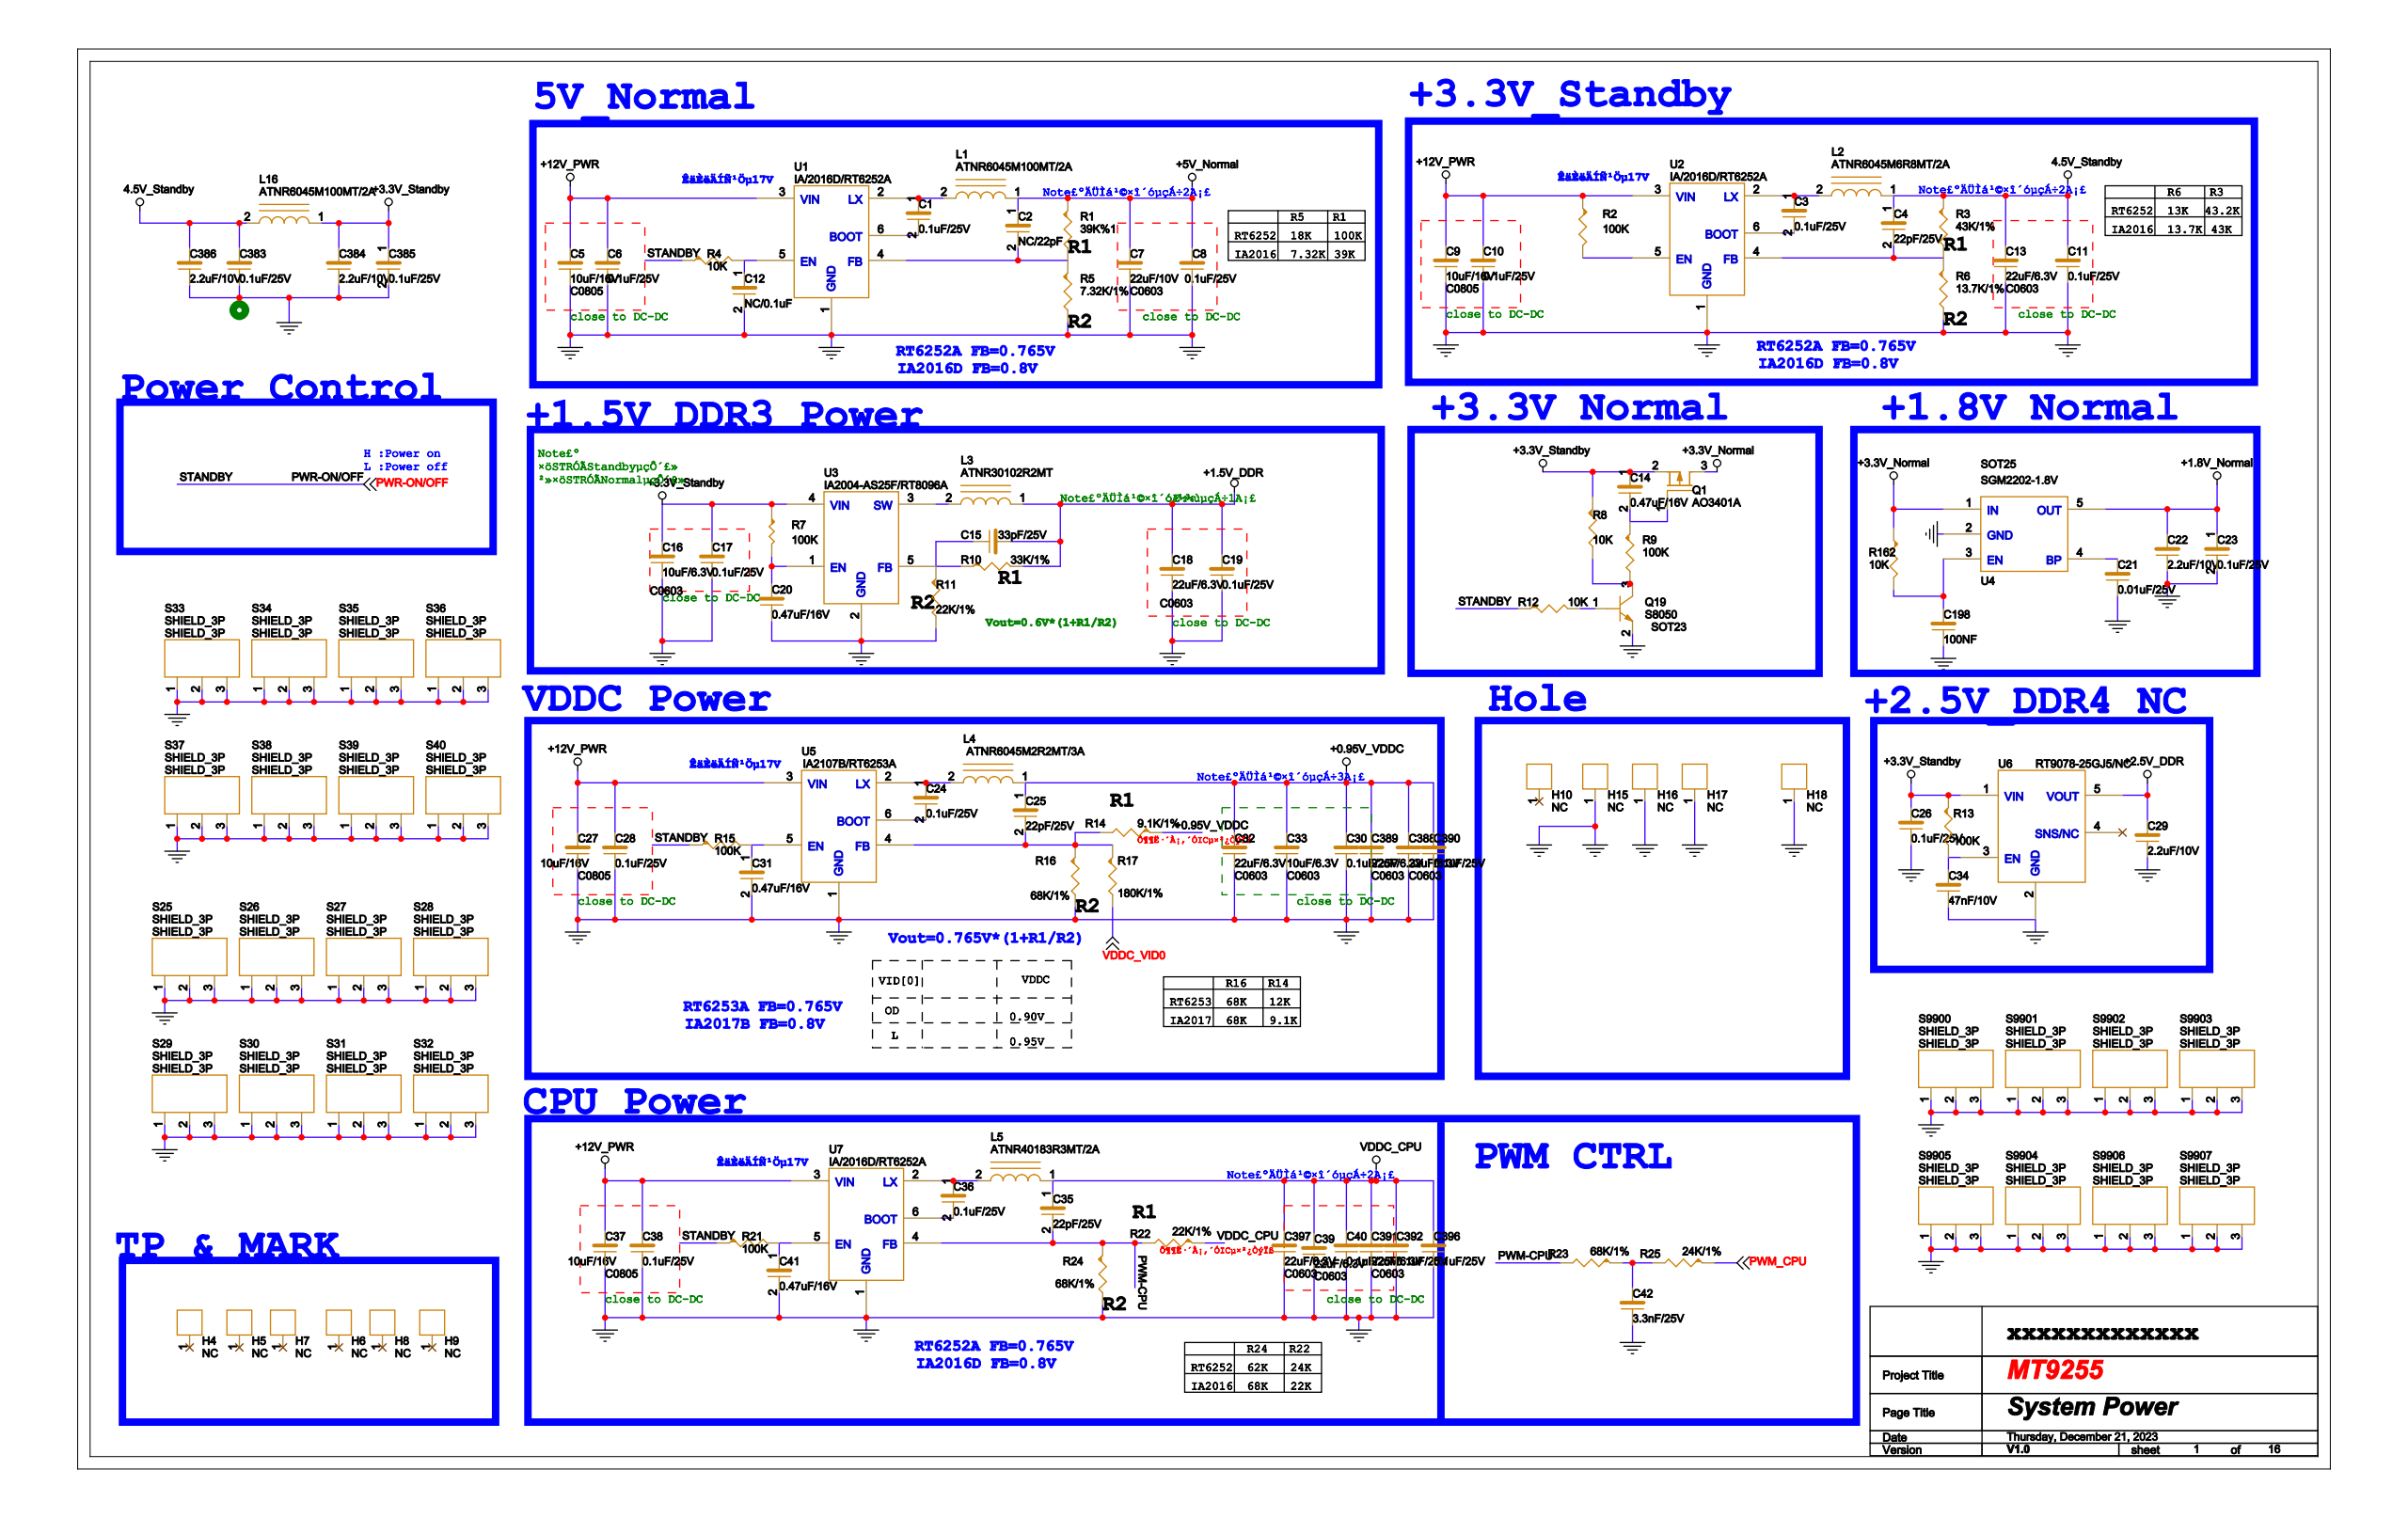Circuit board | Cadence Allegro | 1223 parts | 777 nets | one sheet of the schematic
Parts on this sheet (reference | value | footprint):
C2 | NC/22pF | C0402
C4 | 22pF/25V | C0402
C5 | 10uF/16V | C0805
C6 | 0.1uF/25V | C0402
C7 | 22uF/10V | C0603
C9 | 10uF/16V | C0805
C10 | 0.1uF/25V | C0402
C12 | NC/0.1uF | C0402
C15 | 33pF/25V | C0402
C17 | 0.1uF/25V | C0402
C18 | 22uF/6.3V | C0603
C19 | 0.1uF/25V | C0402
C20 | 0.47uF/16V | C0402
C21 | 0.01uF/25V | C0402
C25 | 22pF/25V | C0402
C26 | 0.1uF/25V | C0402
C27 | 10uF/16V | C0805
C28 | 0.1uF/25V | C0402
C29 | 2.2uF/10V | C0402
C30 | 0.1uF/25V | C0402
C31 | 0.47uF/16V | C0402
C32 | 22uF/6.3V | C0603
C33 | 10uF/6.3V | C0603
C34 | 47nF/10V | C0402
C35 | 22pF/25V | C0402
C36 | 0.1uF/25V | C0402
C37 | 10uF/16V | C0805
C38 | 0.1uF/25V | C0402
C39 | 22uF/6.3V | C0603
C40 | 0.1uF/25V | C0402
C41 | 0.47uF/16V | C0402
C42 | 3.3nF/25V | C0402
C198 | 100NF | C0402
C383 | 0.1uF/25V | C0402
C384 | 2.2uF/10V | C0402
C385 | 0.1uF/25V | C0402
C386 | 2.2uF/10V | C0402
C388 | 22uF/6.3V | C0603
C389 | 22uF/6.3V | C0603
C390 | 0.1uF/25V | C0402
C391 | 22uF/6.3V | C0603
C392 | 0.1uF/25V | C0402
C396 | 0.1uF/25V | C0402
C397 | 22uF/6.3V | C0603
H15 | NC | HOLE_D1D8MM
H16 | NC | HOLE_D1D8MM
H17 | NC | HOLE_D1D8MM
H18 | NC | HOLE_D1D8MM
L1 | ATNR6045M100MT/2A | MWSA0402S
L2 | ATNR6045M6R8MT/2A | MWSA0402S
L3 | ATNR30102R2MT | SMD03X03
L4 | ATNR6045M2R2MT/3A | MWSA0402S
L5 | ATNR40183R3MT/2A | MWSA0402S
L16 | ATNR6045M100MT/2A | MWSA0402S
Q1 | AO3401A | SOT23-100
Q19 | S8050 | SOT23
R3 | 43K/1% | R0402
R4 | 10K | R0402
R6 | 13.7K/1% | R0402
R7 | 100K | R0402
R10 | 33K/1% | R0402
R11 | 22K/1% | R0402
R12 | 10K | R0402
R14 | 9.1K/1% | R0402
R15 | 100K | R0402
R16 | 68K/1% | R0402
R17 | 180K/1% | R0402
R21 | 100K | R0402
R22 | 22K/1% | R0402
R23 | 68K/1% | R0402
R24 | 68K/1% | R0402
R25 | 24K/1% | R0402
R162 | 10K | R0402
S25 | SHIELD_3P | SHIELD_3P
S26 | SHIELD_3P | SHIELD_3P
S27 | SHIELD_3P | SHIELD_3P
S28 | SHIELD_3P | SHIELD_3P
S29 | SHIELD_3P | SHIELD_3P
S30 | SHIELD_3P | SHIELD_3P
S31 | SHIELD_3P | SHIELD_3P
S32 | SHIELD_3P | SHIELD_3P
S33 | SHIELD_3P | SHIELD_3P
S34 | SHIELD_3P | SHIELD_3P
S35 | SHIELD_3P | SHIELD_3P
S36 | SHIELD_3P | SHIELD_3P
S37 | SHIELD_3P | SHIELD_3P
S38 | SHIELD_3P | SHIELD_3P
S39 | SHIELD_3P | SHIELD_3P
S40 | SHIELD_3P | SHIELD_3P
S9900 | SHIELD_3P | SHIELD_3P
S9901 | SHIELD_3P | SHIELD_3P
S9902 | SHIELD_3P | SHIELD_3P
S9903 | SHIELD_3P | SHIELD_3P
S9904 | SHIELD_3P | SHIELD_3P
S9905 | SHIELD_3P | SHIELD_3P
S9906 | SHIELD_3P | SHIELD_3P
S9907 | SHIELD_3P | SHIELD_3P
U1 | IA/2016D/RT6252A | SOT-23-6
U2 | IA/2016D/RT6252A | SOT-23-6
U3 | IA2004-AS25F/RT8096A | SOT25
U4 | SGM2202-1.8V | SOT25
U5 | IA2107B/RT6253A | SOT-23-6
U6 | RT9078-25GJ5/NC | SOT25
U7 | IA/2016D/RT6252A | SOT-23-6
Nets of these parts (net: part-pin ...):
GND: C5-2 C6-2 C7-2 C9-2 C10-2 C12-2 C17-2 C18-2 C19-2 C20-2 C21-2 C26-2 C27-2 C28-2 C29-2 C30-2 C31-2 C32-2 C33-2 C34-2 C37-2 C38-2 C39-2 C40-2 C41-2 C42-2 C198-2 C383-2 C384-2 C385-2 C386-2 C388-2 C389-2 C390-2 C391-2 C392-2 C396-2 C397-2 H15-1 H16-1 H17-1 H18-1 Q19-2 R6-2 R11-2 R16-2 R24-2 S25-1 S25-2 S25-3 S26-1 S26-2 S26-3 S27-1 S27-2 S27-3 S28-1 S28-2 S28-3 S29-1 S29-2 S29-3 S30-1 S30-2 S30-3 S31-1 S31-2 S31-3 S32-1 S32-2 S32-3 S33-1 S33-2 S33-3 S34-1 S34-2 S34-3 S35-1 S35-2 S35-3 S36-1 S36-2 S36-3 S37-1 S37-2 S37-3 S38-1 S38-2 S38-3 S39-1 S39-2 S39-3 S40-1 S40-2 S40-3 S9900-1 S9900-2 S9900-3 S9901-1 S9901-2 S9901-3 S9902-1 S9902-2 S9902-3 S9903-1 S9903-2 S9903-3 S9904-1 S9904-2 S9904-3 S9905-1 S9905-2 S9905-3 S9906-1 S9906-2 S9906-3 S9907-1 S9907-2 S9907-3 U1-1 U2-1 U3-2 U4-2 U5-1 U6-2 U7-1
N21933295: L1-2 U1-2
N21933397: U1-6
N23129752: L4-2 U5-2
N23129850: U5-6
N21934314: L2-2 U2-2
N21934408: U2-6
N23130965: C36-1 L5-2 U7-2
N23131063: C36-2 U7-6
+12V_PWR: C5-1 C6-1 C9-1 C10-1 C27-1 C28-1 C37-1 C38-1 U1-3 U2-3 U5-3 U7-3
4.5V_STANDBY: C4-1 C383-1 C386-1 L2-1 L16-2 R3-1
+3.3V_STANDBY: C17-1 C26-1 C384-1 C385-1 L16-1 Q1-2 R7-1 U3-4 U6-1
+1.5V_DDR: C15-1 C18-1 C19-1 L3-1 R10-2
+0.95V_VDDC: C25-1 C30-1 C32-1 C33-1 C388-1 C389-1 C390-1 L4-1 R14-1
VDDC_CPU: C35-1 C39-1 C40-1 C391-1 C392-1 C396-1 C397-1 L5-1 R22-1
+5V_NORMAL: C2-1 C7-1 L1-1
N21933238: C12-1 R4-2 U1-5
+3.3V_EMMC: Q1-3 R162-1 U4-1
N21624372: Q1-1
N23129706: C31-1 R15-2 U5-5
N23130928: C41-1 R21-2 U7-5
N21625543: C15-2 R10-1 R11-1 U3-5
+1.8V_NORMAL: U4-5
N25966414: C198-1 R162-2 U4-3
N21933368: C2-2 U1-4
N24155290: C20-1 R7-2 U3-1
N25968868: C21-1 U4-4
+2.5V_DDR: C29-1 U6-5
N23129817: C25-2 R14-2 R16-1 R17-1 U5-4
PWM-CPU: C35-2 R22-2 R23-2 R24-1 U7-4
N21934379: C4-2 R3-2 R6-1 U2-4
N23601202: C34-1 U6-3
N23300361: C42-1 R23-1 R25-2
N21625587: L3-2 U3-3
N21625696: Q19-1 R12-2
N21625711: Q19-3
PWR-ON/OFF: R4-1 R12-1 R15-1 R21-1
N21934249: U2-5
VDDC_VID0: R17-2
PWM_CPU: R25-1